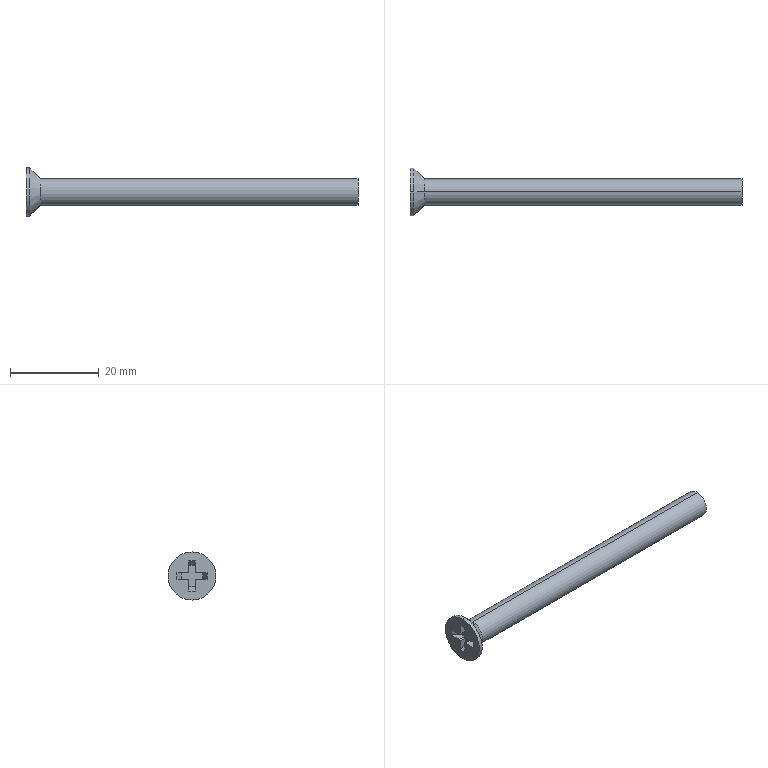Part | SolidWorks | features Cut 2, Revolution 2, Draft 1, Fillet 1, LPattern 1, RevCut 1 | 1 solid | 25 faces | box 75 x 10.9 x 10.9 mm | volume 2225 mm3 | plane 15 | cylinder 8 | cone 2 | commonest cylinder face diameters 0.6 x4 6 x2 10.9 x2
STEP:
#1=CARTESIAN_POINT('',(3.3,0.,-3.));
#2=VERTEX_POINT('',#1);
#3=CARTESIAN_POINT('',(3.3,0.,3.));
#4=VERTEX_POINT('',#3);
#5=CARTESIAN_POINT('',(3.3,0.,0.));
#6=DIRECTION('',(1.,0.,0.));
#7=DIRECTION('',(0.,0.,-1.));
#8=AXIS2_PLACEMENT_3D('',#5,#6,#7);
#9=CIRCLE('',#8,3.);
#10=EDGE_CURVE('',#2,#4,#9,.T.);
#11=ORIENTED_EDGE('',*,*,#10,.T.);
#12=CARTESIAN_POINT('',(75.,0.,3.));
#13=VERTEX_POINT('',#12);
#14=CARTESIAN_POINT('',(4.516,0.,3.));
#15=DIRECTION('',(1.,0.,0.));
#16=VECTOR('',#15,1000.);
#17=LINE('',#14,#16);
#18=EDGE_CURVE('',#4,#13,#17,.T.);
#19=ORIENTED_EDGE('',*,*,#18,.T.);
#20=CARTESIAN_POINT('',(75.,0.,-3.));
#21=VERTEX_POINT('',#20);
#22=CARTESIAN_POINT('',(75.,0.,0.));
#23=DIRECTION('',(1.,0.,0.));
#24=DIRECTION('',(0.,0.,-1.));
#25=AXIS2_PLACEMENT_3D('',#22,#23,#24);
#26=CIRCLE('',#25,3.);
#27=EDGE_CURVE('',#21,#13,#26,.T.);
#28=ORIENTED_EDGE('',*,*,#27,.F.);
#29=CARTESIAN_POINT('',(4.516,0.,-3.));
#30=DIRECTION('',(1.,0.,0.));
#31=VECTOR('',#30,1000.);
#32=LINE('',#29,#31);
#33=EDGE_CURVE('',#2,#21,#32,.T.);
#34=ORIENTED_EDGE('',*,*,#33,.F.);
#35=EDGE_LOOP('',(#11,#19,#28,#34));
#36=FACE_OUTER_BOUND('',#35,.T.);
#37=CARTESIAN_POINT('',(4.516,0.,0.));
#38=DIRECTION('',(1.,0.,0.));
#39=DIRECTION('',(0.,0.,-1.));
#40=AXIS2_PLACEMENT_3D('',#37,#38,#39);
#41=CYLINDRICAL_SURFACE('',#40,3.);
#42=ADVANCED_FACE('',(#36),#41,.T.);
#43=ORIENTED_EDGE('',*,*,#10,.F.);
#44=CARTESIAN_POINT('',(0.85,0.,-5.45));
#45=VERTEX_POINT('',#44);
#46=CARTESIAN_POINT('',(3.3,0.,-3.));
#47=DIRECTION('',(-0.7071,0.,-0.7071));
#48=VECTOR('',#47,1000.);
#49=LINE('',#46,#48);
#50=EDGE_CURVE('',#2,#45,#49,.T.);
#51=ORIENTED_EDGE('',*,*,#50,.T.);
#52=CARTESIAN_POINT('',(0.85,0.,5.45));
#53=VERTEX_POINT('',#52);
#54=CARTESIAN_POINT('',(0.85,0.,0.));
#55=DIRECTION('',(1.,0.,0.));
#56=DIRECTION('',(0.,0.,-1.));
#57=AXIS2_PLACEMENT_3D('',#54,#55,#56);
#58=CIRCLE('',#57,5.45);
#59=EDGE_CURVE('',#45,#53,#58,.T.);
#60=ORIENTED_EDGE('',*,*,#59,.T.);
#61=CARTESIAN_POINT('',(3.3,0.,3.));
#62=DIRECTION('',(-0.7071,0.,0.7071));
#63=VECTOR('',#62,1000.);
#64=LINE('',#61,#63);
#65=EDGE_CURVE('',#4,#53,#64,.T.);
#66=ORIENTED_EDGE('',*,*,#65,.F.);
#67=EDGE_LOOP('',(#43,#51,#60,#66));
#68=FACE_OUTER_BOUND('',#67,.T.);
#69=CARTESIAN_POINT('',(3.3,0.,0.));
#70=DIRECTION('',(-1.,0.,0.));
#71=DIRECTION('',(0.,0.,1.));
#72=AXIS2_PLACEMENT_3D('',#69,#70,#71);
#73=CONICAL_SURFACE('',#72,3.,0.7854);
#74=ADVANCED_FACE('',(#68),#73,.T.);
#75=CARTESIAN_POINT('',(0.,0.,-5.45));
#76=VERTEX_POINT('',#75);
#77=CARTESIAN_POINT('',(0.,0.,5.45));
#78=VERTEX_POINT('',#77);
#79=CARTESIAN_POINT('',(0.,0.,0.));
#80=DIRECTION('',(1.,0.,0.));
#81=DIRECTION('',(0.,0.,-1.));
#82=AXIS2_PLACEMENT_3D('',#79,#80,#81);
#83=CIRCLE('',#82,5.45);
#84=EDGE_CURVE('',#76,#78,#83,.T.);
#85=ORIENTED_EDGE('',*,*,#84,.T.);
#86=CARTESIAN_POINT('',(4.516,0.,5.45));
#87=DIRECTION('',(1.,0.,0.));
#88=VECTOR('',#87,1000.);
#89=LINE('',#86,#88);
#90=EDGE_CURVE('',#78,#53,#89,.T.);
#91=ORIENTED_EDGE('',*,*,#90,.T.);
#92=ORIENTED_EDGE('',*,*,#59,.F.);
#93=CARTESIAN_POINT('',(4.516,0.,-5.45));
#94=DIRECTION('',(1.,0.,0.));
#95=VECTOR('',#94,1000.);
#96=LINE('',#93,#95);
#97=EDGE_CURVE('',#76,#45,#96,.T.);
#98=ORIENTED_EDGE('',*,*,#97,.F.);
#99=EDGE_LOOP('',(#85,#91,#92,#98));
#100=FACE_OUTER_BOUND('',#99,.T.);
#101=CARTESIAN_POINT('',(4.516,0.,0.));
#102=DIRECTION('',(1.,0.,0.));
#103=DIRECTION('',(0.,0.,-1.));
#104=AXIS2_PLACEMENT_3D('',#101,#102,#103);
#105=CYLINDRICAL_SURFACE('',#104,5.45);
#106=ADVANCED_FACE('',(#100),#105,.T.);
#107=ORIENTED_EDGE('',*,*,#84,.F.);
#108=CARTESIAN_POINT('',(0.,0.,0.));
#109=DIRECTION('',(1.,0.,0.));
#110=DIRECTION('',(0.,0.,-1.));
#111=AXIS2_PLACEMENT_3D('',#108,#109,#110);
#112=CIRCLE('',#111,5.45);
#113=EDGE_CURVE('',#78,#76,#112,.T.);
#114=ORIENTED_EDGE('',*,*,#113,.F.);
#115=EDGE_LOOP('',(#107,#114));
#116=FACE_OUTER_BOUND('',#115,.T.);
#117=CARTESIAN_POINT('',(0.,-3.4,-0.68));
#118=VERTEX_POINT('',#117);
#119=CARTESIAN_POINT('',(0.,-0.98,-0.68));
#120=VERTEX_POINT('',#119);
#121=CARTESIAN_POINT('',(0.,-0.68,-0.68));
#122=DIRECTION('',(0.,1.,0.));
#123=VECTOR('',#122,1000.);
#124=LINE('',#121,#123);
#125=EDGE_CURVE('',#118,#120,#124,.T.);
#126=ORIENTED_EDGE('',*,*,#125,.T.);
#127=CARTESIAN_POINT('',(0.,-0.68,-0.98));
#128=VERTEX_POINT('',#127);
#129=CARTESIAN_POINT('',(0.,-0.98,-0.98));
#130=DIRECTION('',(-1.,0.,0.));
#131=DIRECTION('',(0.,0.,1.));
#132=AXIS2_PLACEMENT_3D('',#129,#130,#131);
#133=CIRCLE('',#132,0.3);
#134=EDGE_CURVE('',#120,#128,#133,.T.);
#135=ORIENTED_EDGE('',*,*,#134,.T.);
#136=CARTESIAN_POINT('',(0.,-0.68,-3.4));
#137=VERTEX_POINT('',#136);
#138=CARTESIAN_POINT('',(0.,-0.68,-0.68));
#139=DIRECTION('',(0.,0.,-1.));
#140=VECTOR('',#139,1000.);
#141=LINE('',#138,#140);
#142=EDGE_CURVE('',#128,#137,#141,.T.);
#143=ORIENTED_EDGE('',*,*,#142,.T.);
#144=CARTESIAN_POINT('',(0.,0.68,-3.4));
#145=VERTEX_POINT('',#144);
#146=CARTESIAN_POINT('',(0.,0.68,-3.4));
#147=DIRECTION('',(0.,1.,0.));
#148=VECTOR('',#147,1000.);
#149=LINE('',#146,#148);
#150=EDGE_CURVE('',#137,#145,#149,.T.);
#151=ORIENTED_EDGE('',*,*,#150,.T.);
#152=CARTESIAN_POINT('',(0.,0.68,-0.98));
#153=VERTEX_POINT('',#152);
#154=CARTESIAN_POINT('',(0.,0.68,-0.68));
#155=DIRECTION('',(0.,0.,1.));
#156=VECTOR('',#155,1000.);
#157=LINE('',#154,#156);
#158=EDGE_CURVE('',#145,#153,#157,.T.);
#159=ORIENTED_EDGE('',*,*,#158,.T.);
#160=CARTESIAN_POINT('',(0.,0.98,-0.68));
#161=VERTEX_POINT('',#160);
#162=CARTESIAN_POINT('',(0.,0.98,-0.98));
#163=DIRECTION('',(-1.,0.,0.));
#164=DIRECTION('',(0.,0.,1.));
#165=AXIS2_PLACEMENT_3D('',#162,#163,#164);
#166=CIRCLE('',#165,0.3);
#167=EDGE_CURVE('',#153,#161,#166,.T.);
#168=ORIENTED_EDGE('',*,*,#167,.T.);
#169=CARTESIAN_POINT('',(0.,3.4,-0.68));
#170=VERTEX_POINT('',#169);
#171=CARTESIAN_POINT('',(0.,0.68,-0.68));
#172=DIRECTION('',(0.,1.,0.));
#173=VECTOR('',#172,1000.);
#174=LINE('',#171,#173);
#175=EDGE_CURVE('',#161,#170,#174,.T.);
#176=ORIENTED_EDGE('',*,*,#175,.T.);
#177=CARTESIAN_POINT('',(0.,3.4,0.68));
#178=VERTEX_POINT('',#177);
#179=CARTESIAN_POINT('',(0.,3.4,-0.68));
#180=DIRECTION('',(0.,0.,1.));
#181=VECTOR('',#180,1000.);
#182=LINE('',#179,#181);
#183=EDGE_CURVE('',#170,#178,#182,.T.);
#184=ORIENTED_EDGE('',*,*,#183,.T.);
#185=CARTESIAN_POINT('',(0.,0.98,0.68));
#186=VERTEX_POINT('',#185);
#187=CARTESIAN_POINT('',(0.,0.68,0.68));
#188=DIRECTION('',(0.,-1.,0.));
#189=VECTOR('',#188,1000.);
#190=LINE('',#187,#189);
#191=EDGE_CURVE('',#178,#186,#190,.T.);
#192=ORIENTED_EDGE('',*,*,#191,.T.);
#193=CARTESIAN_POINT('',(0.,0.68,0.98));
#194=VERTEX_POINT('',#193);
#195=CARTESIAN_POINT('',(0.,0.98,0.98));
#196=DIRECTION('',(-1.,0.,0.));
#197=DIRECTION('',(0.,0.,1.));
#198=AXIS2_PLACEMENT_3D('',#195,#196,#197);
#199=CIRCLE('',#198,0.3);
#200=EDGE_CURVE('',#186,#194,#199,.T.);
#201=ORIENTED_EDGE('',*,*,#200,.T.);
#202=CARTESIAN_POINT('',(0.,0.68,3.4));
#203=VERTEX_POINT('',#202);
#204=CARTESIAN_POINT('',(0.,0.68,0.68));
#205=DIRECTION('',(0.,0.,1.));
#206=VECTOR('',#205,1000.);
#207=LINE('',#204,#206);
#208=EDGE_CURVE('',#194,#203,#207,.T.);
#209=ORIENTED_EDGE('',*,*,#208,.T.);
#210=CARTESIAN_POINT('',(0.,-0.68,3.4));
#211=VERTEX_POINT('',#210);
#212=CARTESIAN_POINT('',(0.,0.68,3.4));
#213=DIRECTION('',(0.,-1.,0.));
#214=VECTOR('',#213,1000.);
#215=LINE('',#212,#214);
#216=EDGE_CURVE('',#203,#211,#215,.T.);
#217=ORIENTED_EDGE('',*,*,#216,.T.);
#218=CARTESIAN_POINT('',(0.,-0.68,0.98));
#219=VERTEX_POINT('',#218);
#220=CARTESIAN_POINT('',(0.,-0.68,0.68));
#221=DIRECTION('',(0.,0.,-1.));
#222=VECTOR('',#221,1000.);
#223=LINE('',#220,#222);
#224=EDGE_CURVE('',#211,#219,#223,.T.);
#225=ORIENTED_EDGE('',*,*,#224,.T.);
#226=CARTESIAN_POINT('',(0.,-0.98,0.68));
#227=VERTEX_POINT('',#226);
#228=CARTESIAN_POINT('',(0.,-0.98,0.98));
#229=DIRECTION('',(-1.,0.,0.));
#230=DIRECTION('',(0.,0.,1.));
#231=AXIS2_PLACEMENT_3D('',#228,#229,#230);
#232=CIRCLE('',#231,0.3);
#233=EDGE_CURVE('',#219,#227,#232,.T.);
#234=ORIENTED_EDGE('',*,*,#233,.T.);
#235=CARTESIAN_POINT('',(0.,-3.4,0.68));
#236=VERTEX_POINT('',#235);
#237=CARTESIAN_POINT('',(0.,-0.68,0.68));
#238=DIRECTION('',(0.,-1.,0.));
#239=VECTOR('',#238,1000.);
#240=LINE('',#237,#239);
#241=EDGE_CURVE('',#227,#236,#240,.T.);
#242=ORIENTED_EDGE('',*,*,#241,.T.);
#243=CARTESIAN_POINT('',(0.,-3.4,-0.68));
#244=DIRECTION('',(0.,0.,-1.));
#245=VECTOR('',#244,1000.);
#246=LINE('',#243,#245);
#247=EDGE_CURVE('',#236,#118,#246,.T.);
#248=ORIENTED_EDGE('',*,*,#247,.T.);
#249=EDGE_LOOP('',(#126,#135,#143,#151,#159,#168,#176,#184,#192,#201,#209,#217,#225,#234,#242,#248));
#250=FACE_BOUND('',#249,.T.);
#251=CARTESIAN_POINT('',(0.,5.45,0.));
#252=DIRECTION('',(-1.,0.,0.));
#253=DIRECTION('',(0.,0.,1.));
#254=AXIS2_PLACEMENT_3D('',#251,#252,#253);
#255=PLANE('',#254);
#256=ADVANCED_FACE('',(#116,#250),#255,.T.);
#257=ORIENTED_EDGE('',*,*,#27,.T.);
#258=CARTESIAN_POINT('',(75.,0.,0.));
#259=DIRECTION('',(1.,0.,0.));
#260=DIRECTION('',(0.,0.,-1.));
#261=AXIS2_PLACEMENT_3D('',#258,#259,#260);
#262=CIRCLE('',#261,3.);
#263=EDGE_CURVE('',#13,#21,#262,.T.);
#264=ORIENTED_EDGE('',*,*,#263,.T.);
#265=EDGE_LOOP('',(#257,#264));
#266=FACE_OUTER_BOUND('',#265,.T.);
#267=CARTESIAN_POINT('',(75.,3.,0.));
#268=DIRECTION('',(1.,0.,0.));
#269=DIRECTION('',(0.,0.,-1.));
#270=AXIS2_PLACEMENT_3D('',#267,#268,#269);
#271=PLANE('',#270);
#272=ADVANCED_FACE('',(#266),#271,.T.);
#273=ORIENTED_EDGE('',*,*,#90,.F.);
#274=ORIENTED_EDGE('',*,*,#113,.T.);
#275=ORIENTED_EDGE('',*,*,#97,.T.);
#276=CARTESIAN_POINT('',(0.85,0.,0.));
#277=DIRECTION('',(1.,0.,0.));
#278=DIRECTION('',(0.,0.,-1.));
#279=AXIS2_PLACEMENT_3D('',#276,#277,#278);
#280=CIRCLE('',#279,5.45);
#281=EDGE_CURVE('',#53,#45,#280,.T.);
#282=ORIENTED_EDGE('',*,*,#281,.F.);
#283=EDGE_LOOP('',(#273,#274,#275,#282));
#284=FACE_OUTER_BOUND('',#283,.T.);
#285=CARTESIAN_POINT('',(4.516,0.,0.));
#286=DIRECTION('',(1.,0.,0.));
#287=DIRECTION('',(0.,0.,-1.));
#288=AXIS2_PLACEMENT_3D('',#285,#286,#287);
#289=CYLINDRICAL_SURFACE('',#288,5.45);
#290=ADVANCED_FACE('',(#284),#289,.T.);
#291=ORIENTED_EDGE('',*,*,#50,.F.);
#292=CARTESIAN_POINT('',(3.3,0.,0.));
#293=DIRECTION('',(1.,0.,0.));
#294=DIRECTION('',(0.,0.,-1.));
#295=AXIS2_PLACEMENT_3D('',#292,#293,#294);
#296=CIRCLE('',#295,3.);
#297=EDGE_CURVE('',#4,#2,#296,.T.);
#298=ORIENTED_EDGE('',*,*,#297,.F.);
#299=ORIENTED_EDGE('',*,*,#65,.T.);
#300=ORIENTED_EDGE('',*,*,#281,.T.);
#301=EDGE_LOOP('',(#291,#298,#299,#300));
#302=FACE_OUTER_BOUND('',#301,.T.);
#303=CARTESIAN_POINT('',(3.3,0.,0.));
#304=DIRECTION('',(-1.,0.,0.));
#305=DIRECTION('',(0.,0.,1.));
#306=AXIS2_PLACEMENT_3D('',#303,#304,#305);
#307=CONICAL_SURFACE('',#306,3.,0.7854);
#308=ADVANCED_FACE('',(#302),#307,.T.);
#309=ORIENTED_EDGE('',*,*,#18,.F.);
#310=ORIENTED_EDGE('',*,*,#297,.T.);
#311=ORIENTED_EDGE('',*,*,#33,.T.);
#312=ORIENTED_EDGE('',*,*,#263,.F.);
#313=EDGE_LOOP('',(#309,#310,#311,#312));
#314=FACE_OUTER_BOUND('',#313,.T.);
#315=CARTESIAN_POINT('',(4.516,0.,0.));
#316=DIRECTION('',(1.,0.,0.));
#317=DIRECTION('',(0.,0.,-1.));
#318=AXIS2_PLACEMENT_3D('',#315,#316,#317);
#319=CYLINDRICAL_SURFACE('',#318,3.);
#320=ADVANCED_FACE('',(#314),#319,.T.);
#321=ORIENTED_EDGE('',*,*,#208,.F.);
#322=CARTESIAN_POINT('',(1.65,0.68,0.98));
#323=VERTEX_POINT('',#322);
#324=CARTESIAN_POINT('',(1.65,0.68,0.98));
#325=DIRECTION('',(1.,0.,0.));
#326=VECTOR('',#325,1000.);
#327=LINE('',#324,#326);
#328=EDGE_CURVE('',#194,#323,#327,.T.);
#329=ORIENTED_EDGE('',*,*,#328,.T.);
#330=CARTESIAN_POINT('',(1.65,0.68,2.447));
#331=VERTEX_POINT('',#330);
#332=CARTESIAN_POINT('',(1.65,0.68,0.68));
#333=DIRECTION('',(0.,0.,1.));
#334=VECTOR('',#333,1000.);
#335=LINE('',#332,#334);
#336=EDGE_CURVE('',#323,#331,#335,.T.);
#337=ORIENTED_EDGE('',*,*,#336,.T.);
#338=CARTESIAN_POINT('',(0.,0.68,3.4));
#339=DIRECTION('',(-0.866,0.,0.5));
#340=VECTOR('',#339,1000.);
#341=LINE('',#338,#340);
#342=EDGE_CURVE('',#331,#203,#341,.T.);
#343=ORIENTED_EDGE('',*,*,#342,.T.);
#344=EDGE_LOOP('',(#321,#329,#337,#343));
#345=FACE_OUTER_BOUND('',#344,.T.);
#346=CARTESIAN_POINT('',(1.65,0.68,0.68));
#347=DIRECTION('',(0.,-1.,0.));
#348=DIRECTION('',(0.,0.,-1.));
#349=AXIS2_PLACEMENT_3D('',#346,#347,#348);
#350=PLANE('',#349);
#351=ADVANCED_FACE('',(#345),#350,.T.);
#352=ORIENTED_EDGE('',*,*,#216,.F.);
#353=ORIENTED_EDGE('',*,*,#342,.F.);
#354=CARTESIAN_POINT('',(1.65,-0.68,2.447));
#355=VERTEX_POINT('',#354);
#356=CARTESIAN_POINT('',(1.65,0.68,2.447));
#357=DIRECTION('',(0.,-1.,0.));
#358=VECTOR('',#357,1000.);
#359=LINE('',#356,#358);
#360=EDGE_CURVE('',#331,#355,#359,.T.);
#361=ORIENTED_EDGE('',*,*,#360,.T.);
#362=CARTESIAN_POINT('',(2.415,-0.68,2.006));
#363=DIRECTION('',(-0.866,0.,0.5));
#364=VECTOR('',#363,1000.);
#365=LINE('',#362,#364);
#366=EDGE_CURVE('',#355,#211,#365,.T.);
#367=ORIENTED_EDGE('',*,*,#366,.T.);
#368=EDGE_LOOP('',(#352,#353,#361,#367));
#369=FACE_OUTER_BOUND('',#368,.T.);
#370=CARTESIAN_POINT('',(0.,0.68,3.4));
#371=DIRECTION('',(-0.5,0.,-0.866));
#372=DIRECTION('',(-0.866,0.,0.5));
#373=AXIS2_PLACEMENT_3D('',#370,#371,#372);
#374=PLANE('',#373);
#375=ADVANCED_FACE('',(#369),#374,.T.);
#376=CARTESIAN_POINT('',(1.65,-0.68,0.98));
#377=VERTEX_POINT('',#376);
#378=CARTESIAN_POINT('',(1.65,-0.68,0.68));
#379=DIRECTION('',(0.,0.,-1.));
#380=VECTOR('',#379,1000.);
#381=LINE('',#378,#380);
#382=EDGE_CURVE('',#355,#377,#381,.T.);
#383=ORIENTED_EDGE('',*,*,#382,.T.);
#384=CARTESIAN_POINT('',(1.65,-0.68,0.98));
#385=DIRECTION('',(-1.,0.,0.));
#386=VECTOR('',#385,1000.);
#387=LINE('',#384,#386);
#388=EDGE_CURVE('',#377,#219,#387,.T.);
#389=ORIENTED_EDGE('',*,*,#388,.T.);
#390=ORIENTED_EDGE('',*,*,#224,.F.);
#391=ORIENTED_EDGE('',*,*,#366,.F.);
#392=EDGE_LOOP('',(#383,#389,#390,#391));
#393=FACE_OUTER_BOUND('',#392,.T.);
#394=CARTESIAN_POINT('',(1.65,-0.68,0.68));
#395=DIRECTION('',(0.,1.,0.));
#396=DIRECTION('',(0.,0.,1.));
#397=AXIS2_PLACEMENT_3D('',#394,#395,#396);
#398=PLANE('',#397);
#399=ADVANCED_FACE('',(#393),#398,.T.);
#400=ORIENTED_EDGE('',*,*,#241,.F.);
#401=CARTESIAN_POINT('',(1.65,-0.98,0.68));
#402=VERTEX_POINT('',#401);
#403=CARTESIAN_POINT('',(1.65,-0.98,0.68));
#404=DIRECTION('',(1.,0.,0.));
#405=VECTOR('',#404,1000.);
#406=LINE('',#403,#405);
#407=EDGE_CURVE('',#227,#402,#406,.T.);
#408=ORIENTED_EDGE('',*,*,#407,.T.);
#409=CARTESIAN_POINT('',(1.65,-2.447,0.68));
#410=VERTEX_POINT('',#409);
#411=CARTESIAN_POINT('',(1.65,-0.68,0.68));
#412=DIRECTION('',(0.,-1.,0.));
#413=VECTOR('',#412,1000.);
#414=LINE('',#411,#413);
#415=EDGE_CURVE('',#402,#410,#414,.T.);
#416=ORIENTED_EDGE('',*,*,#415,.T.);
#417=CARTESIAN_POINT('',(0.,-3.4,0.68));
#418=DIRECTION('',(-0.866,-0.5,0.));
#419=VECTOR('',#418,1000.);
#420=LINE('',#417,#419);
#421=EDGE_CURVE('',#410,#236,#420,.T.);
#422=ORIENTED_EDGE('',*,*,#421,.T.);
#423=EDGE_LOOP('',(#400,#408,#416,#422));
#424=FACE_OUTER_BOUND('',#423,.T.);
#425=CARTESIAN_POINT('',(1.65,-0.68,0.68));
#426=DIRECTION('',(0.,0.,-1.));
#427=DIRECTION('',(0.,1.,0.));
#428=AXIS2_PLACEMENT_3D('',#425,#426,#427);
#429=PLANE('',#428);
#430=ADVANCED_FACE('',(#424),#429,.T.);
#431=ORIENTED_EDGE('',*,*,#247,.F.);
#432=ORIENTED_EDGE('',*,*,#421,.F.);
#433=CARTESIAN_POINT('',(1.65,-2.447,-0.68));
#434=VERTEX_POINT('',#433);
#435=CARTESIAN_POINT('',(1.65,-2.447,-0.68));
#436=DIRECTION('',(0.,0.,-1.));
#437=VECTOR('',#436,1000.);
#438=LINE('',#435,#437);
#439=EDGE_CURVE('',#410,#434,#438,.T.);
#440=ORIENTED_EDGE('',*,*,#439,.T.);
#441=CARTESIAN_POINT('',(2.415,-2.006,-0.68));
#442=DIRECTION('',(-0.866,-0.5,0.));
#443=VECTOR('',#442,1000.);
#444=LINE('',#441,#443);
#445=EDGE_CURVE('',#434,#118,#444,.T.);
#446=ORIENTED_EDGE('',*,*,#445,.T.);
#447=EDGE_LOOP('',(#431,#432,#440,#446));
#448=FACE_OUTER_BOUND('',#447,.T.);
#449=CARTESIAN_POINT('',(0.,-3.4,-0.68));
#450=DIRECTION('',(-0.5,0.866,0.));
#451=DIRECTION('',(-0.866,-0.5,0.));
#452=AXIS2_PLACEMENT_3D('',#449,#450,#451);
#453=PLANE('',#452);
#454=ADVANCED_FACE('',(#448),#453,.T.);
#455=CARTESIAN_POINT('',(1.65,-0.98,-0.68));
#456=VERTEX_POINT('',#455);
#457=CARTESIAN_POINT('',(1.65,-0.68,-0.68));
#458=DIRECTION('',(0.,1.,0.));
#459=VECTOR('',#458,1000.);
#460=LINE('',#457,#459);
#461=EDGE_CURVE('',#434,#456,#460,.T.);
#462=ORIENTED_EDGE('',*,*,#461,.T.);
#463=CARTESIAN_POINT('',(1.65,-0.98,-0.68));
#464=DIRECTION('',(-1.,0.,0.));
#465=VECTOR('',#464,1000.);
#466=LINE('',#463,#465);
#467=EDGE_CURVE('',#456,#120,#466,.T.);
#468=ORIENTED_EDGE('',*,*,#467,.T.);
#469=ORIENTED_EDGE('',*,*,#125,.F.);
#470=ORIENTED_EDGE('',*,*,#445,.F.);
#471=EDGE_LOOP('',(#462,#468,#469,#470));
#472=FACE_OUTER_BOUND('',#471,.T.);
#473=CARTESIAN_POINT('',(1.65,-0.68,-0.68));
#474=DIRECTION('',(0.,0.,1.));
#475=DIRECTION('',(1.,0.,0.));
#476=AXIS2_PLACEMENT_3D('',#473,#474,#475);
#477=PLANE('',#476);
#478=ADVANCED_FACE('',(#472),#477,.T.);
#479=ORIENTED_EDGE('',*,*,#142,.F.);
#480=CARTESIAN_POINT('',(1.65,-0.68,-0.98));
#481=VERTEX_POINT('',#480);
#482=CARTESIAN_POINT('',(1.65,-0.68,-0.98));
#483=DIRECTION('',(1.,0.,0.));
#484=VECTOR('',#483,1000.);
#485=LINE('',#482,#484);
#486=EDGE_CURVE('',#128,#481,#485,.T.);
#487=ORIENTED_EDGE('',*,*,#486,.T.);
#488=CARTESIAN_POINT('',(1.65,-0.68,-2.447));
#489=VERTEX_POINT('',#488);
#490=CARTESIAN_POINT('',(1.65,-0.68,-0.68));
#491=DIRECTION('',(0.,0.,-1.));
#492=VECTOR('',#491,1000.);
#493=LINE('',#490,#492);
#494=EDGE_CURVE('',#481,#489,#493,.T.);
#495=ORIENTED_EDGE('',*,*,#494,.T.);
#496=CARTESIAN_POINT('',(0.,-0.68,-3.4));
#497=DIRECTION('',(-0.866,0.,-0.5));
#498=VECTOR('',#497,1000.);
#499=LINE('',#496,#498);
#500=EDGE_CURVE('',#489,#137,#499,.T.);
#501=ORIENTED_EDGE('',*,*,#500,.T.);
#502=EDGE_LOOP('',(#479,#487,#495,#501));
#503=FACE_OUTER_BOUND('',#502,.T.);
#504=CARTESIAN_POINT('',(1.65,-0.68,-0.68));
#505=DIRECTION('',(0.,1.,0.));
#506=DIRECTION('',(0.,0.,1.));
#507=AXIS2_PLACEMENT_3D('',#504,#505,#506);
#508=PLANE('',#507);
#509=ADVANCED_FACE('',(#503),#508,.T.);
#510=ORIENTED_EDGE('',*,*,#150,.F.);
#511=ORIENTED_EDGE('',*,*,#500,.F.);
#512=CARTESIAN_POINT('',(1.65,0.68,-2.447));
#513=VERTEX_POINT('',#512);
#514=CARTESIAN_POINT('',(1.65,0.68,-2.447));
#515=DIRECTION('',(0.,1.,0.));
#516=VECTOR('',#515,1000.);
#517=LINE('',#514,#516);
#518=EDGE_CURVE('',#489,#513,#517,.T.);
#519=ORIENTED_EDGE('',*,*,#518,.T.);
#520=CARTESIAN_POINT('',(2.415,0.68,-2.006));
#521=DIRECTION('',(-0.866,0.,-0.5));
#522=VECTOR('',#521,1000.);
#523=LINE('',#520,#522);
#524=EDGE_CURVE('',#513,#145,#523,.T.);
#525=ORIENTED_EDGE('',*,*,#524,.T.);
#526=EDGE_LOOP('',(#510,#511,#519,#525));
#527=FACE_OUTER_BOUND('',#526,.T.);
#528=CARTESIAN_POINT('',(0.,0.68,-3.4));
#529=DIRECTION('',(-0.5,0.,0.866));
#530=DIRECTION('',(0.866,0.,0.5));
#531=AXIS2_PLACEMENT_3D('',#528,#529,#530);
#532=PLANE('',#531);
#533=ADVANCED_FACE('',(#527),#532,.T.);
#534=CARTESIAN_POINT('',(1.65,0.68,-0.98));
#535=VERTEX_POINT('',#534);
#536=CARTESIAN_POINT('',(1.65,0.68,-0.68));
#537=DIRECTION('',(0.,0.,1.));
#538=VECTOR('',#537,1000.);
#539=LINE('',#536,#538);
#540=EDGE_CURVE('',#513,#535,#539,.T.);
#541=ORIENTED_EDGE('',*,*,#540,.T.);
#542=CARTESIAN_POINT('',(1.65,0.68,-0.98));
#543=DIRECTION('',(-1.,0.,0.));
#544=VECTOR('',#543,1000.);
#545=LINE('',#542,#544);
#546=EDGE_CURVE('',#535,#153,#545,.T.);
#547=ORIENTED_EDGE('',*,*,#546,.T.);
#548=ORIENTED_EDGE('',*,*,#158,.F.);
#549=ORIENTED_EDGE('',*,*,#524,.F.);
#550=EDGE_LOOP('',(#541,#547,#548,#549));
#551=FACE_OUTER_BOUND('',#550,.T.);
#552=CARTESIAN_POINT('',(1.65,0.68,-0.68));
#553=DIRECTION('',(0.,-1.,0.));
#554=DIRECTION('',(0.,0.,-1.));
#555=AXIS2_PLACEMENT_3D('',#552,#553,#554);
#556=PLANE('',#555);
#557=ADVANCED_FACE('',(#551),#556,.T.);
#558=ORIENTED_EDGE('',*,*,#175,.F.);
#559=CARTESIAN_POINT('',(1.65,0.98,-0.68));
#560=VERTEX_POINT('',#559);
#561=CARTESIAN_POINT('',(1.65,0.98,-0.68));
#562=DIRECTION('',(1.,0.,0.));
#563=VECTOR('',#562,1000.);
#564=LINE('',#561,#563);
#565=EDGE_CURVE('',#161,#560,#564,.T.);
#566=ORIENTED_EDGE('',*,*,#565,.T.);
#567=CARTESIAN_POINT('',(1.65,2.447,-0.68));
#568=VERTEX_POINT('',#567);
#569=CARTESIAN_POINT('',(1.65,0.68,-0.68));
#570=DIRECTION('',(0.,1.,0.));
#571=VECTOR('',#570,1000.);
#572=LINE('',#569,#571);
#573=EDGE_CURVE('',#560,#568,#572,.T.);
#574=ORIENTED_EDGE('',*,*,#573,.T.);
#575=CARTESIAN_POINT('',(0.,3.4,-0.68));
#576=DIRECTION('',(-0.866,0.5,0.));
#577=VECTOR('',#576,1000.);
#578=LINE('',#575,#577);
#579=EDGE_CURVE('',#568,#170,#578,.T.);
#580=ORIENTED_EDGE('',*,*,#579,.T.);
#581=EDGE_LOOP('',(#558,#566,#574,#580));
#582=FACE_OUTER_BOUND('',#581,.T.);
#583=CARTESIAN_POINT('',(1.65,0.68,-0.68));
#584=DIRECTION('',(0.,0.,1.));
#585=DIRECTION('',(1.,0.,0.));
#586=AXIS2_PLACEMENT_3D('',#583,#584,#585);
#587=PLANE('',#586);
#588=ADVANCED_FACE('',(#582),#587,.T.);
#589=ORIENTED_EDGE('',*,*,#183,.F.);
#590=ORIENTED_EDGE('',*,*,#579,.F.);
#591=CARTESIAN_POINT('',(1.65,2.447,0.68));
#592=VERTEX_POINT('',#591);
#593=CARTESIAN_POINT('',(1.65,2.447,-0.68));
#594=DIRECTION('',(0.,0.,1.));
#595=VECTOR('',#594,1000.);
#596=LINE('',#593,#595);
#597=EDGE_CURVE('',#568,#592,#596,.T.);
#598=ORIENTED_EDGE('',*,*,#597,.T.);
#599=CARTESIAN_POINT('',(2.415,2.006,0.68));
#600=DIRECTION('',(-0.866,0.5,0.));
#601=VECTOR('',#600,1000.);
#602=LINE('',#599,#601);
#603=EDGE_CURVE('',#592,#178,#602,.T.);
#604=ORIENTED_EDGE('',*,*,#603,.T.);
#605=EDGE_LOOP('',(#589,#590,#598,#604));
#606=FACE_OUTER_BOUND('',#605,.T.);
#607=CARTESIAN_POINT('',(0.,3.4,-0.68));
#608=DIRECTION('',(-0.5,-0.866,0.));
#609=DIRECTION('',(0.866,-0.5,0.));
#610=AXIS2_PLACEMENT_3D('',#607,#608,#609);
#611=PLANE('',#610);
#612=ADVANCED_FACE('',(#606),#611,.T.);
#613=CARTESIAN_POINT('',(1.65,0.98,0.68));
#614=VERTEX_POINT('',#613);
#615=CARTESIAN_POINT('',(1.65,0.68,0.68));
#616=DIRECTION('',(0.,-1.,0.));
#617=VECTOR('',#616,1000.);
#618=LINE('',#615,#617);
#619=EDGE_CURVE('',#592,#614,#618,.T.);
#620=ORIENTED_EDGE('',*,*,#619,.T.);
#621=CARTESIAN_POINT('',(1.65,0.98,0.68));
#622=DIRECTION('',(-1.,0.,0.));
#623=VECTOR('',#622,1000.);
#624=LINE('',#621,#623);
#625=EDGE_CURVE('',#614,#186,#624,.T.);
#626=ORIENTED_EDGE('',*,*,#625,.T.);
#627=ORIENTED_EDGE('',*,*,#191,.F.);
#628=ORIENTED_EDGE('',*,*,#603,.F.);
#629=EDGE_LOOP('',(#620,#626,#627,#628));
#630=FACE_OUTER_BOUND('',#629,.T.);
#631=CARTESIAN_POINT('',(1.65,0.68,0.68));
#632=DIRECTION('',(0.,0.,-1.));
#633=DIRECTION('',(0.,1.,0.));
#634=AXIS2_PLACEMENT_3D('',#631,#632,#633);
#635=PLANE('',#634);
#636=ADVANCED_FACE('',(#630),#635,.T.);
#637=ORIENTED_EDGE('',*,*,#336,.F.);
#638=CARTESIAN_POINT('',(1.65,0.98,0.98));
#639=DIRECTION('',(1.,0.,0.));
#640=DIRECTION('',(0.,0.,-1.));
#641=AXIS2_PLACEMENT_3D('',#638,#639,#640);
#642=CIRCLE('',#641,0.3);
#643=EDGE_CURVE('',#323,#614,#642,.T.);
#644=ORIENTED_EDGE('',*,*,#643,.T.);
#645=ORIENTED_EDGE('',*,*,#619,.F.);
#646=ORIENTED_EDGE('',*,*,#597,.F.);
#647=ORIENTED_EDGE('',*,*,#573,.F.);
#648=CARTESIAN_POINT('',(1.65,0.98,-0.98));
#649=DIRECTION('',(1.,0.,0.));
#650=DIRECTION('',(0.,0.,-1.));
#651=AXIS2_PLACEMENT_3D('',#648,#649,#650);
#652=CIRCLE('',#651,0.3);
#653=EDGE_CURVE('',#560,#535,#652,.T.);
#654=ORIENTED_EDGE('',*,*,#653,.T.);
#655=ORIENTED_EDGE('',*,*,#540,.F.);
#656=ORIENTED_EDGE('',*,*,#518,.F.);
#657=ORIENTED_EDGE('',*,*,#494,.F.);
#658=CARTESIAN_POINT('',(1.65,-0.98,-0.98));
#659=DIRECTION('',(1.,0.,0.));
#660=DIRECTION('',(0.,0.,-1.));
#661=AXIS2_PLACEMENT_3D('',#658,#659,#660);
#662=CIRCLE('',#661,0.3);
#663=EDGE_CURVE('',#481,#456,#662,.T.);
#664=ORIENTED_EDGE('',*,*,#663,.T.);
#665=ORIENTED_EDGE('',*,*,#461,.F.);
#666=ORIENTED_EDGE('',*,*,#439,.F.);
#667=ORIENTED_EDGE('',*,*,#415,.F.);
#668=CARTESIAN_POINT('',(1.65,-0.98,0.98));
#669=DIRECTION('',(1.,0.,0.));
#670=DIRECTION('',(0.,0.,-1.));
#671=AXIS2_PLACEMENT_3D('',#668,#669,#670);
#672=CIRCLE('',#671,0.3);
#673=EDGE_CURVE('',#402,#377,#672,.T.);
#674=ORIENTED_EDGE('',*,*,#673,.T.);
#675=ORIENTED_EDGE('',*,*,#382,.F.);
#676=ORIENTED_EDGE('',*,*,#360,.F.);
#677=EDGE_LOOP('',(#637,#644,#645,#646,#647,#654,#655,#656,#657,#664,#665,#666,#667,#674,#675,#676));
#678=FACE_OUTER_BOUND('',#677,.T.);
#679=CARTESIAN_POINT('',(1.65,0.68,0.68));
#680=DIRECTION('',(1.,0.,0.));
#681=DIRECTION('',(0.,0.,-1.));
#682=AXIS2_PLACEMENT_3D('',#679,#680,#681);
#683=PLANE('',#682);
#684=ADVANCED_FACE('',(#678),#683,.F.);
#685=ORIENTED_EDGE('',*,*,#663,.F.);
#686=ORIENTED_EDGE('',*,*,#486,.F.);
#687=ORIENTED_EDGE('',*,*,#134,.F.);
#688=ORIENTED_EDGE('',*,*,#467,.F.);
#689=EDGE_LOOP('',(#685,#686,#687,#688));
#690=FACE_OUTER_BOUND('',#689,.T.);
#691=CARTESIAN_POINT('',(1.65,-0.98,-0.98));
#692=DIRECTION('',(-1.,0.,0.));
#693=DIRECTION('',(0.,0.,1.));
#694=AXIS2_PLACEMENT_3D('',#691,#692,#693);
#695=CYLINDRICAL_SURFACE('',#694,0.3);
#696=ADVANCED_FACE('',(#690),#695,.T.);
#697=ORIENTED_EDGE('',*,*,#673,.F.);
#698=ORIENTED_EDGE('',*,*,#407,.F.);
#699=ORIENTED_EDGE('',*,*,#233,.F.);
#700=ORIENTED_EDGE('',*,*,#388,.F.);
#701=EDGE_LOOP('',(#697,#698,#699,#700));
#702=FACE_OUTER_BOUND('',#701,.T.);
#703=CARTESIAN_POINT('',(1.65,-0.98,0.98));
#704=DIRECTION('',(-1.,0.,0.));
#705=DIRECTION('',(0.,0.,1.));
#706=AXIS2_PLACEMENT_3D('',#703,#704,#705);
#707=CYLINDRICAL_SURFACE('',#706,0.3);
#708=ADVANCED_FACE('',(#702),#707,.T.);
#709=ORIENTED_EDGE('',*,*,#653,.F.);
#710=ORIENTED_EDGE('',*,*,#565,.F.);
#711=ORIENTED_EDGE('',*,*,#167,.F.);
#712=ORIENTED_EDGE('',*,*,#546,.F.);
#713=EDGE_LOOP('',(#709,#710,#711,#712));
#714=FACE_OUTER_BOUND('',#713,.T.);
#715=CARTESIAN_POINT('',(1.65,0.98,-0.98));
#716=DIRECTION('',(-1.,0.,0.));
#717=DIRECTION('',(0.,0.,1.));
#718=AXIS2_PLACEMENT_3D('',#715,#716,#717);
#719=CYLINDRICAL_SURFACE('',#718,0.3);
#720=ADVANCED_FACE('',(#714),#719,.T.);
#721=ORIENTED_EDGE('',*,*,#643,.F.);
#722=ORIENTED_EDGE('',*,*,#328,.F.);
#723=ORIENTED_EDGE('',*,*,#200,.F.);
#724=ORIENTED_EDGE('',*,*,#625,.F.);
#725=EDGE_LOOP('',(#721,#722,#723,#724));
#726=FACE_OUTER_BOUND('',#725,.T.);
#727=CARTESIAN_POINT('',(1.65,0.98,0.98));
#728=DIRECTION('',(-1.,0.,0.));
#729=DIRECTION('',(0.,0.,1.));
#730=AXIS2_PLACEMENT_3D('',#727,#728,#729);
#731=CYLINDRICAL_SURFACE('',#730,0.3);
#732=ADVANCED_FACE('',(#726),#731,.T.);
#733=CLOSED_SHELL('',(#42,#74,#106,#256,#272,#290,#308,#320,#351,#375,#399,#430,#454,#478,#509,#533,#557,#588,#612,#636,#684,#696,#708,#720,#732));
#734=MANIFOLD_SOLID_BREP('',#733);
#735=CARTESIAN_POINT('',(0.,0.,0.));
#736=DIRECTION('',(0.,0.,1.));
#737=DIRECTION('',(1.,0.,0.));
#738=AXIS2_PLACEMENT_3D('',#735,#736,#737);
#739=(LENGTH_UNIT()NAMED_UNIT(*)SI_UNIT(.MILLI.,.METRE.));
#740=UNCERTAINTY_MEASURE_WITH_UNIT(LENGTH_MEASURE(0.00001),#739,'','');
#741=(NAMED_UNIT(*)PLANE_ANGLE_UNIT()SI_UNIT($,.RADIAN.));
#742=(NAMED_UNIT(*)SI_UNIT($,.STERADIAN.)SOLID_ANGLE_UNIT());
#743=(GEOMETRIC_REPRESENTATION_CONTEXT(3)GLOBAL_UNCERTAINTY_ASSIGNED_CONTEXT((#740))GLOBAL_UNIT_ASSIGNED_CONTEXT((#739,#741,#742))REPRESENTATION_CONTEXT('',''));
#744=ADVANCED_BREP_SHAPE_REPRESENTATION('',(#734,#738),#743);